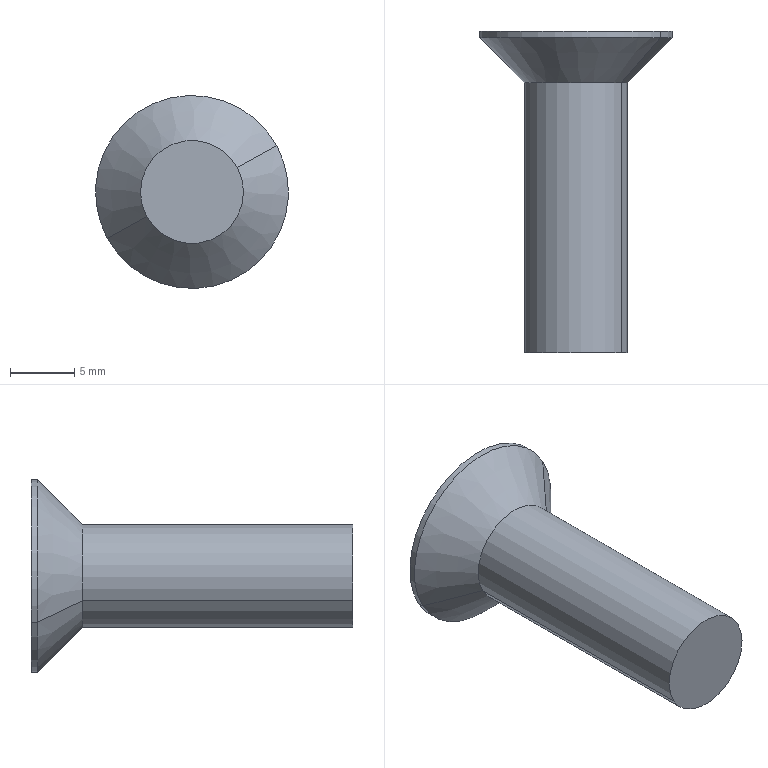Part | NX | features BREP 1 | 1 solid | 21 faces | box 15 x 25 x 15 mm | volume 1509 mm3 | plane 15 | cylinder 4 | cone 2 | commonest cylinder face diameters 8 x2 15 x2
STEP:
#1=CARTESIAN_POINT('',(3.51,31.308,1.918));
#2=VERTEX_POINT('',#1);
#3=CARTESIAN_POINT('',(-3.51,31.308,-1.918));
#4=VERTEX_POINT('',#3);
#5=CARTESIAN_POINT('',(0.,31.308,0.));
#6=DIRECTION('',(0.,-1.,0.));
#7=DIRECTION('',(1.,0.,0.));
#8=AXIS2_PLACEMENT_3D('',#5,#6,#7);
#9=CIRCLE('',#8,4.);
#10=EDGE_CURVE('',#2,#4,#9,.T.);
#11=ORIENTED_EDGE('',*,*,#10,.F.);
#12=CARTESIAN_POINT('',(3.51,52.308,1.918));
#13=VERTEX_POINT('',#12);
#14=CARTESIAN_POINT('',(3.51,41.808,1.918));
#15=DIRECTION('',(0.,-1.,0.));
#16=VECTOR('',#15,1000.);
#17=LINE('',#14,#16);
#18=EDGE_CURVE('',#2,#13,#17,.F.);
#19=ORIENTED_EDGE('',*,*,#18,.T.);
#20=CARTESIAN_POINT('',(-3.51,52.308,-1.918));
#21=VERTEX_POINT('',#20);
#22=CARTESIAN_POINT('',(0.,52.308,0.));
#23=DIRECTION('',(0.,1.,0.));
#24=DIRECTION('',(1.,0.,0.));
#25=AXIS2_PLACEMENT_3D('',#22,#23,#24);
#26=CIRCLE('',#25,4.);
#27=EDGE_CURVE('',#21,#13,#26,.T.);
#28=ORIENTED_EDGE('',*,*,#27,.F.);
#29=CARTESIAN_POINT('',(-3.51,41.808,-1.918));
#30=DIRECTION('',(0.,-1.,0.));
#31=VECTOR('',#30,1000.);
#32=LINE('',#29,#31);
#33=EDGE_CURVE('',#4,#21,#32,.F.);
#34=ORIENTED_EDGE('',*,*,#33,.F.);
#35=EDGE_LOOP('',(#11,#19,#28,#34));
#36=FACE_BOUND('',#35,.T.);
#37=CARTESIAN_POINT('',(0.,43.808,0.));
#38=DIRECTION('',(0.,-1.,0.));
#39=DIRECTION('',(0.8776,0.,0.4794));
#40=AXIS2_PLACEMENT_3D('',#37,#38,#39);
#41=CYLINDRICAL_SURFACE('',#40,4.);
#42=ADVANCED_FACE('',(#36),#41,.T.);
#43=CARTESIAN_POINT('',(0.,31.308,0.));
#44=DIRECTION('',(0.,-1.,0.));
#45=DIRECTION('',(1.,0.,0.));
#46=AXIS2_PLACEMENT_3D('',#43,#44,#45);
#47=CIRCLE('',#46,4.);
#48=EDGE_CURVE('',#4,#2,#47,.T.);
#49=ORIENTED_EDGE('',*,*,#48,.F.);
#50=ORIENTED_EDGE('',*,*,#33,.T.);
#51=CARTESIAN_POINT('',(0.,52.308,0.));
#52=DIRECTION('',(0.,1.,0.));
#53=DIRECTION('',(1.,0.,0.));
#54=AXIS2_PLACEMENT_3D('',#51,#52,#53);
#55=CIRCLE('',#54,4.);
#56=EDGE_CURVE('',#13,#21,#55,.T.);
#57=ORIENTED_EDGE('',*,*,#56,.F.);
#58=ORIENTED_EDGE('',*,*,#18,.F.);
#59=EDGE_LOOP('',(#49,#50,#57,#58));
#60=FACE_BOUND('',#59,.T.);
#61=CARTESIAN_POINT('',(0.,43.808,0.));
#62=DIRECTION('',(0.,-1.,0.));
#63=DIRECTION('',(0.8776,0.,0.4794));
#64=AXIS2_PLACEMENT_3D('',#61,#62,#63);
#65=CYLINDRICAL_SURFACE('',#64,4.);
#66=ADVANCED_FACE('',(#60),#65,.T.);
#67=ORIENTED_EDGE('',*,*,#27,.T.);
#68=CARTESIAN_POINT('',(6.582,55.808,3.596));
#69=VERTEX_POINT('',#68);
#70=CARTESIAN_POINT('',(5.046,54.058,2.757));
#71=DIRECTION('',(0.6205,0.7071,0.339));
#72=VECTOR('',#71,1000.);
#73=LINE('',#70,#72);
#74=EDGE_CURVE('',#69,#13,#73,.F.);
#75=ORIENTED_EDGE('',*,*,#74,.F.);
#76=CARTESIAN_POINT('',(-6.582,55.808,-3.596));
#77=VERTEX_POINT('',#76);
#78=CARTESIAN_POINT('',(0.,55.808,0.));
#79=DIRECTION('',(0.,-1.,0.));
#80=DIRECTION('',(1.,0.,0.));
#81=AXIS2_PLACEMENT_3D('',#78,#79,#80);
#82=CIRCLE('',#81,7.5);
#83=EDGE_CURVE('',#69,#77,#82,.T.);
#84=ORIENTED_EDGE('',*,*,#83,.T.);
#85=CARTESIAN_POINT('',(-5.046,54.058,-2.757));
#86=DIRECTION('',(-0.6205,0.7071,-0.339));
#87=VECTOR('',#86,1000.);
#88=LINE('',#85,#87);
#89=EDGE_CURVE('',#77,#21,#88,.F.);
#90=ORIENTED_EDGE('',*,*,#89,.T.);
#91=EDGE_LOOP('',(#67,#75,#84,#90));
#92=FACE_BOUND('',#91,.T.);
#93=CARTESIAN_POINT('',(0.,52.308,0.));
#94=DIRECTION('',(0.,1.,0.));
#95=DIRECTION('',(0.8776,0.,0.4794));
#96=AXIS2_PLACEMENT_3D('',#93,#94,#95);
#97=CONICAL_SURFACE('',#96,4.,0.7854);
#98=ADVANCED_FACE('',(#92),#97,.T.);
#99=ORIENTED_EDGE('',*,*,#56,.T.);
#100=ORIENTED_EDGE('',*,*,#89,.F.);
#101=CARTESIAN_POINT('',(0.,55.808,0.));
#102=DIRECTION('',(0.,-1.,0.));
#103=DIRECTION('',(1.,0.,0.));
#104=AXIS2_PLACEMENT_3D('',#101,#102,#103);
#105=CIRCLE('',#104,7.5);
#106=EDGE_CURVE('',#77,#69,#105,.T.);
#107=ORIENTED_EDGE('',*,*,#106,.T.);
#108=ORIENTED_EDGE('',*,*,#74,.T.);
#109=EDGE_LOOP('',(#99,#100,#107,#108));
#110=FACE_BOUND('',#109,.T.);
#111=CARTESIAN_POINT('',(0.,52.308,0.));
#112=DIRECTION('',(0.,1.,0.));
#113=DIRECTION('',(0.8776,0.,0.4794));
#114=AXIS2_PLACEMENT_3D('',#111,#112,#113);
#115=CONICAL_SURFACE('',#114,4.,0.7854);
#116=ADVANCED_FACE('',(#110),#115,.T.);
#117=ORIENTED_EDGE('',*,*,#83,.F.);
#118=CARTESIAN_POINT('',(6.582,56.308,3.596));
#119=VERTEX_POINT('',#118);
#120=CARTESIAN_POINT('',(6.582,56.058,3.596));
#121=DIRECTION('',(0.,-1.,0.));
#122=VECTOR('',#121,1000.);
#123=LINE('',#120,#122);
#124=EDGE_CURVE('',#69,#119,#123,.F.);
#125=ORIENTED_EDGE('',*,*,#124,.T.);
#126=CARTESIAN_POINT('',(-6.582,56.308,-3.596));
#127=VERTEX_POINT('',#126);
#128=CARTESIAN_POINT('',(0.,56.308,0.));
#129=DIRECTION('',(0.,-1.,0.));
#130=DIRECTION('',(1.,0.,0.));
#131=AXIS2_PLACEMENT_3D('',#128,#129,#130);
#132=CIRCLE('',#131,7.5);
#133=EDGE_CURVE('',#119,#127,#132,.T.);
#134=ORIENTED_EDGE('',*,*,#133,.T.);
#135=CARTESIAN_POINT('',(-6.582,56.058,-3.596));
#136=DIRECTION('',(0.,-1.,0.));
#137=VECTOR('',#136,1000.);
#138=LINE('',#135,#137);
#139=EDGE_CURVE('',#77,#127,#138,.F.);
#140=ORIENTED_EDGE('',*,*,#139,.F.);
#141=EDGE_LOOP('',(#117,#125,#134,#140));
#142=FACE_BOUND('',#141,.T.);
#143=CARTESIAN_POINT('',(0.,43.808,0.));
#144=DIRECTION('',(0.,-1.,0.));
#145=DIRECTION('',(0.8776,0.,0.4794));
#146=AXIS2_PLACEMENT_3D('',#143,#144,#145);
#147=CYLINDRICAL_SURFACE('',#146,7.5);
#148=ADVANCED_FACE('',(#142),#147,.T.);
#149=ORIENTED_EDGE('',*,*,#106,.F.);
#150=ORIENTED_EDGE('',*,*,#139,.T.);
#151=CARTESIAN_POINT('',(0.,56.308,0.));
#152=DIRECTION('',(0.,-1.,0.));
#153=DIRECTION('',(1.,0.,0.));
#154=AXIS2_PLACEMENT_3D('',#151,#152,#153);
#155=CIRCLE('',#154,7.5);
#156=EDGE_CURVE('',#127,#119,#155,.T.);
#157=ORIENTED_EDGE('',*,*,#156,.T.);
#158=ORIENTED_EDGE('',*,*,#124,.F.);
#159=EDGE_LOOP('',(#149,#150,#157,#158));
#160=FACE_BOUND('',#159,.T.);
#161=CARTESIAN_POINT('',(0.,43.808,0.));
#162=DIRECTION('',(0.,-1.,0.));
#163=DIRECTION('',(0.8776,0.,0.4794));
#164=AXIS2_PLACEMENT_3D('',#161,#162,#163);
#165=CYLINDRICAL_SURFACE('',#164,7.5);
#166=ADVANCED_FACE('',(#160),#165,.T.);
#167=ORIENTED_EDGE('',*,*,#10,.T.);
#168=ORIENTED_EDGE('',*,*,#48,.T.);
#169=EDGE_LOOP('',(#167,#168));
#170=FACE_BOUND('',#169,.T.);
#171=CARTESIAN_POINT('',(4.,31.308,0.));
#172=DIRECTION('',(0.,-1.,0.));
#173=DIRECTION('',(1.,0.,0.));
#174=AXIS2_PLACEMENT_3D('',#171,#172,#173);
#175=PLANE('',#174);
#176=ADVANCED_FACE('',(#170),#175,.T.);
#177=CARTESIAN_POINT('',(1.,56.308,2.));
#178=VERTEX_POINT('',#177);
#179=CARTESIAN_POINT('',(1.,56.308,1.));
#180=VERTEX_POINT('',#179);
#181=CARTESIAN_POINT('',(1.,56.308,1.5));
#182=DIRECTION('',(0.,0.,-1.));
#183=VECTOR('',#182,1000.);
#184=LINE('',#181,#183);
#185=EDGE_CURVE('',#178,#180,#184,.T.);
#186=ORIENTED_EDGE('',*,*,#185,.F.);
#187=CARTESIAN_POINT('',(-1.,56.308,2.));
#188=VERTEX_POINT('',#187);
#189=CARTESIAN_POINT('',(0.,56.308,2.));
#190=DIRECTION('',(-1.,0.,0.));
#191=VECTOR('',#190,1000.);
#192=LINE('',#189,#191);
#193=EDGE_CURVE('',#178,#188,#192,.T.);
#194=ORIENTED_EDGE('',*,*,#193,.T.);
#195=CARTESIAN_POINT('',(-1.,56.308,1.));
#196=VERTEX_POINT('',#195);
#197=CARTESIAN_POINT('',(-1.,56.308,1.5));
#198=DIRECTION('',(0.,0.,1.));
#199=VECTOR('',#198,1000.);
#200=LINE('',#197,#199);
#201=EDGE_CURVE('',#196,#188,#200,.T.);
#202=ORIENTED_EDGE('',*,*,#201,.F.);
#203=CARTESIAN_POINT('',(-2.,56.308,1.));
#204=VERTEX_POINT('',#203);
#205=CARTESIAN_POINT('',(-1.5,56.308,1.));
#206=DIRECTION('',(-1.,0.,0.));
#207=VECTOR('',#206,1000.);
#208=LINE('',#205,#207);
#209=EDGE_CURVE('',#196,#204,#208,.T.);
#210=ORIENTED_EDGE('',*,*,#209,.T.);
#211=CARTESIAN_POINT('',(-2.,56.308,-1.));
#212=VERTEX_POINT('',#211);
#213=CARTESIAN_POINT('',(-2.,56.308,0.));
#214=DIRECTION('',(0.,0.,1.));
#215=VECTOR('',#214,1000.);
#216=LINE('',#213,#215);
#217=EDGE_CURVE('',#212,#204,#216,.T.);
#218=ORIENTED_EDGE('',*,*,#217,.F.);
#219=CARTESIAN_POINT('',(-1.,56.308,-1.));
#220=VERTEX_POINT('',#219);
#221=CARTESIAN_POINT('',(-1.5,56.308,-1.));
#222=DIRECTION('',(1.,0.,0.));
#223=VECTOR('',#222,1000.);
#224=LINE('',#221,#223);
#225=EDGE_CURVE('',#212,#220,#224,.T.);
#226=ORIENTED_EDGE('',*,*,#225,.T.);
#227=CARTESIAN_POINT('',(-1.,56.308,-2.));
#228=VERTEX_POINT('',#227);
#229=CARTESIAN_POINT('',(-1.,56.308,-1.5));
#230=DIRECTION('',(0.,0.,1.));
#231=VECTOR('',#230,1000.);
#232=LINE('',#229,#231);
#233=EDGE_CURVE('',#228,#220,#232,.T.);
#234=ORIENTED_EDGE('',*,*,#233,.F.);
#235=CARTESIAN_POINT('',(1.,56.308,-2.));
#236=VERTEX_POINT('',#235);
#237=CARTESIAN_POINT('',(0.,56.308,-2.));
#238=DIRECTION('',(1.,0.,0.));
#239=VECTOR('',#238,1000.);
#240=LINE('',#237,#239);
#241=EDGE_CURVE('',#228,#236,#240,.T.);
#242=ORIENTED_EDGE('',*,*,#241,.T.);
#243=CARTESIAN_POINT('',(1.,56.308,-1.));
#244=VERTEX_POINT('',#243);
#245=CARTESIAN_POINT('',(1.,56.308,-1.5));
#246=DIRECTION('',(0.,0.,-1.));
#247=VECTOR('',#246,1000.);
#248=LINE('',#245,#247);
#249=EDGE_CURVE('',#244,#236,#248,.T.);
#250=ORIENTED_EDGE('',*,*,#249,.F.);
#251=CARTESIAN_POINT('',(2.,56.308,-1.));
#252=VERTEX_POINT('',#251);
#253=CARTESIAN_POINT('',(1.5,56.308,-1.));
#254=DIRECTION('',(1.,0.,0.));
#255=VECTOR('',#254,1000.);
#256=LINE('',#253,#255);
#257=EDGE_CURVE('',#244,#252,#256,.T.);
#258=ORIENTED_EDGE('',*,*,#257,.T.);
#259=CARTESIAN_POINT('',(2.,56.308,1.));
#260=VERTEX_POINT('',#259);
#261=CARTESIAN_POINT('',(2.,56.308,0.));
#262=DIRECTION('',(0.,0.,-1.));
#263=VECTOR('',#262,1000.);
#264=LINE('',#261,#263);
#265=EDGE_CURVE('',#260,#252,#264,.T.);
#266=ORIENTED_EDGE('',*,*,#265,.F.);
#267=CARTESIAN_POINT('',(1.5,56.308,1.));
#268=DIRECTION('',(-1.,0.,0.));
#269=VECTOR('',#268,1000.);
#270=LINE('',#267,#269);
#271=EDGE_CURVE('',#260,#180,#270,.T.);
#272=ORIENTED_EDGE('',*,*,#271,.T.);
#273=EDGE_LOOP('',(#186,#194,#202,#210,#218,#226,#234,#242,#250,#258,#266,#272));
#274=FACE_BOUND('',#273,.T.);
#275=ORIENTED_EDGE('',*,*,#133,.F.);
#276=ORIENTED_EDGE('',*,*,#156,.F.);
#277=EDGE_LOOP('',(#275,#276));
#278=FACE_BOUND('',#277,.T.);
#279=CARTESIAN_POINT('',(0.,56.308,0.));
#280=DIRECTION('',(0.,-1.,0.));
#281=DIRECTION('',(1.,0.,0.));
#282=AXIS2_PLACEMENT_3D('',#279,#280,#281);
#283=PLANE('',#282);
#284=ADVANCED_FACE('',(#274,#278),#283,.F.);
#285=CARTESIAN_POINT('',(-1.,55.508,2.));
#286=VERTEX_POINT('',#285);
#287=CARTESIAN_POINT('',(-1.,55.908,2.));
#288=DIRECTION('',(0.,-1.,0.));
#289=VECTOR('',#288,1000.);
#290=LINE('',#287,#289);
#291=EDGE_CURVE('',#188,#286,#290,.T.);
#292=ORIENTED_EDGE('',*,*,#291,.F.);
#293=ORIENTED_EDGE('',*,*,#193,.F.);
#294=CARTESIAN_POINT('',(1.,55.508,2.));
#295=VERTEX_POINT('',#294);
#296=CARTESIAN_POINT('',(1.,55.908,2.));
#297=DIRECTION('',(0.,-1.,0.));
#298=VECTOR('',#297,1000.);
#299=LINE('',#296,#298);
#300=EDGE_CURVE('',#178,#295,#299,.T.);
#301=ORIENTED_EDGE('',*,*,#300,.T.);
#302=CARTESIAN_POINT('',(0.,55.508,2.));
#303=DIRECTION('',(-1.,0.,0.));
#304=VECTOR('',#303,1000.);
#305=LINE('',#302,#304);
#306=EDGE_CURVE('',#295,#286,#305,.T.);
#307=ORIENTED_EDGE('',*,*,#306,.T.);
#308=EDGE_LOOP('',(#292,#293,#301,#307));
#309=FACE_BOUND('',#308,.T.);
#310=CARTESIAN_POINT('',(1.,56.308,2.));
#311=DIRECTION('',(0.,0.,1.));
#312=DIRECTION('',(-1.,0.,0.));
#313=AXIS2_PLACEMENT_3D('',#310,#311,#312);
#314=PLANE('',#313);
#315=ADVANCED_FACE('',(#309),#314,.F.);
#316=CARTESIAN_POINT('',(-1.,55.508,1.));
#317=VERTEX_POINT('',#316);
#318=CARTESIAN_POINT('',(-1.,55.908,1.));
#319=DIRECTION('',(0.,-1.,0.));
#320=VECTOR('',#319,1000.);
#321=LINE('',#318,#320);
#322=EDGE_CURVE('',#196,#317,#321,.T.);
#323=ORIENTED_EDGE('',*,*,#322,.F.);
#324=ORIENTED_EDGE('',*,*,#201,.T.);
#325=ORIENTED_EDGE('',*,*,#291,.T.);
#326=CARTESIAN_POINT('',(-1.,55.508,1.5));
#327=DIRECTION('',(0.,0.,1.));
#328=VECTOR('',#327,1000.);
#329=LINE('',#326,#328);
#330=EDGE_CURVE('',#317,#286,#329,.T.);
#331=ORIENTED_EDGE('',*,*,#330,.F.);
#332=EDGE_LOOP('',(#323,#324,#325,#331));
#333=FACE_BOUND('',#332,.T.);
#334=CARTESIAN_POINT('',(-1.,56.308,-2.));
#335=DIRECTION('',(1.,0.,0.));
#336=DIRECTION('',(0.,0.,1.));
#337=AXIS2_PLACEMENT_3D('',#334,#335,#336);
#338=PLANE('',#337);
#339=ADVANCED_FACE('',(#333),#338,.T.);
#340=CARTESIAN_POINT('',(-2.,55.508,1.));
#341=VERTEX_POINT('',#340);
#342=CARTESIAN_POINT('',(-2.,55.908,1.));
#343=DIRECTION('',(0.,-1.,0.));
#344=VECTOR('',#343,1000.);
#345=LINE('',#342,#344);
#346=EDGE_CURVE('',#204,#341,#345,.T.);
#347=ORIENTED_EDGE('',*,*,#346,.F.);
#348=ORIENTED_EDGE('',*,*,#209,.F.);
#349=ORIENTED_EDGE('',*,*,#322,.T.);
#350=CARTESIAN_POINT('',(-1.5,55.508,1.));
#351=DIRECTION('',(-1.,0.,0.));
#352=VECTOR('',#351,1000.);
#353=LINE('',#350,#352);
#354=EDGE_CURVE('',#317,#341,#353,.T.);
#355=ORIENTED_EDGE('',*,*,#354,.T.);
#356=EDGE_LOOP('',(#347,#348,#349,#355));
#357=FACE_BOUND('',#356,.T.);
#358=CARTESIAN_POINT('',(-1.,56.308,1.));
#359=DIRECTION('',(0.,0.,1.));
#360=DIRECTION('',(-1.,0.,0.));
#361=AXIS2_PLACEMENT_3D('',#358,#359,#360);
#362=PLANE('',#361);
#363=ADVANCED_FACE('',(#357),#362,.F.);
#364=CARTESIAN_POINT('',(-2.,55.508,-1.));
#365=VERTEX_POINT('',#364);
#366=CARTESIAN_POINT('',(-2.,55.908,-1.));
#367=DIRECTION('',(0.,-1.,0.));
#368=VECTOR('',#367,1000.);
#369=LINE('',#366,#368);
#370=EDGE_CURVE('',#212,#365,#369,.T.);
#371=ORIENTED_EDGE('',*,*,#370,.F.);
#372=ORIENTED_EDGE('',*,*,#217,.T.);
#373=ORIENTED_EDGE('',*,*,#346,.T.);
#374=CARTESIAN_POINT('',(-2.,55.508,0.));
#375=DIRECTION('',(0.,0.,1.));
#376=VECTOR('',#375,1000.);
#377=LINE('',#374,#376);
#378=EDGE_CURVE('',#365,#341,#377,.T.);
#379=ORIENTED_EDGE('',*,*,#378,.F.);
#380=EDGE_LOOP('',(#371,#372,#373,#379));
#381=FACE_BOUND('',#380,.T.);
#382=CARTESIAN_POINT('',(-2.,56.308,-1.));
#383=DIRECTION('',(1.,0.,0.));
#384=DIRECTION('',(0.,0.,1.));
#385=AXIS2_PLACEMENT_3D('',#382,#383,#384);
#386=PLANE('',#385);
#387=ADVANCED_FACE('',(#381),#386,.T.);
#388=CARTESIAN_POINT('',(-1.,55.508,-1.));
#389=VERTEX_POINT('',#388);
#390=CARTESIAN_POINT('',(-1.,55.908,-1.));
#391=DIRECTION('',(0.,-1.,0.));
#392=VECTOR('',#391,1000.);
#393=LINE('',#390,#392);
#394=EDGE_CURVE('',#220,#389,#393,.T.);
#395=ORIENTED_EDGE('',*,*,#394,.F.);
#396=ORIENTED_EDGE('',*,*,#225,.F.);
#397=ORIENTED_EDGE('',*,*,#370,.T.);
#398=CARTESIAN_POINT('',(-1.5,55.508,-1.));
#399=DIRECTION('',(1.,0.,0.));
#400=VECTOR('',#399,1000.);
#401=LINE('',#398,#400);
#402=EDGE_CURVE('',#365,#389,#401,.T.);
#403=ORIENTED_EDGE('',*,*,#402,.T.);
#404=EDGE_LOOP('',(#395,#396,#397,#403));
#405=FACE_BOUND('',#404,.T.);
#406=CARTESIAN_POINT('',(1.,56.308,-1.));
#407=DIRECTION('',(0.,0.,-1.));
#408=DIRECTION('',(1.,0.,0.));
#409=AXIS2_PLACEMENT_3D('',#406,#407,#408);
#410=PLANE('',#409);
#411=ADVANCED_FACE('',(#405),#410,.F.);
#412=CARTESIAN_POINT('',(-1.,55.508,-2.));
#413=VERTEX_POINT('',#412);
#414=CARTESIAN_POINT('',(-1.,55.908,-2.));
#415=DIRECTION('',(0.,-1.,0.));
#416=VECTOR('',#415,1000.);
#417=LINE('',#414,#416);
#418=EDGE_CURVE('',#228,#413,#417,.T.);
#419=ORIENTED_EDGE('',*,*,#418,.F.);
#420=ORIENTED_EDGE('',*,*,#233,.T.);
#421=ORIENTED_EDGE('',*,*,#394,.T.);
#422=CARTESIAN_POINT('',(-1.,55.508,-1.5));
#423=DIRECTION('',(0.,0.,1.));
#424=VECTOR('',#423,1000.);
#425=LINE('',#422,#424);
#426=EDGE_CURVE('',#413,#389,#425,.T.);
#427=ORIENTED_EDGE('',*,*,#426,.F.);
#428=EDGE_LOOP('',(#419,#420,#421,#427));
#429=FACE_BOUND('',#428,.T.);
#430=CARTESIAN_POINT('',(-1.,56.308,-2.));
#431=DIRECTION('',(1.,0.,0.));
#432=DIRECTION('',(0.,0.,1.));
#433=AXIS2_PLACEMENT_3D('',#430,#431,#432);
#434=PLANE('',#433);
#435=ADVANCED_FACE('',(#429),#434,.T.);
#436=CARTESIAN_POINT('',(1.,55.508,-2.));
#437=VERTEX_POINT('',#436);
#438=CARTESIAN_POINT('',(1.,55.908,-2.));
#439=DIRECTION('',(0.,-1.,0.));
#440=VECTOR('',#439,1000.);
#441=LINE('',#438,#440);
#442=EDGE_CURVE('',#236,#437,#441,.T.);
#443=ORIENTED_EDGE('',*,*,#442,.F.);
#444=ORIENTED_EDGE('',*,*,#241,.F.);
#445=ORIENTED_EDGE('',*,*,#418,.T.);
#446=CARTESIAN_POINT('',(0.,55.508,-2.));
#447=DIRECTION('',(1.,0.,0.));
#448=VECTOR('',#447,1000.);
#449=LINE('',#446,#448);
#450=EDGE_CURVE('',#413,#437,#449,.T.);
#451=ORIENTED_EDGE('',*,*,#450,.T.);
#452=EDGE_LOOP('',(#443,#444,#445,#451));
#453=FACE_BOUND('',#452,.T.);
#454=CARTESIAN_POINT('',(-1.,56.308,-2.));
#455=DIRECTION('',(0.,0.,-1.));
#456=DIRECTION('',(1.,0.,0.));
#457=AXIS2_PLACEMENT_3D('',#454,#455,#456);
#458=PLANE('',#457);
#459=ADVANCED_FACE('',(#453),#458,.F.);
#460=CARTESIAN_POINT('',(1.,55.508,-1.));
#461=VERTEX_POINT('',#460);
#462=CARTESIAN_POINT('',(1.,55.908,-1.));
#463=DIRECTION('',(0.,-1.,0.));
#464=VECTOR('',#463,1000.);
#465=LINE('',#462,#464);
#466=EDGE_CURVE('',#244,#461,#465,.T.);
#467=ORIENTED_EDGE('',*,*,#466,.F.);
#468=ORIENTED_EDGE('',*,*,#249,.T.);
#469=ORIENTED_EDGE('',*,*,#442,.T.);
#470=CARTESIAN_POINT('',(1.,55.508,-1.5));
#471=DIRECTION('',(0.,0.,-1.));
#472=VECTOR('',#471,1000.);
#473=LINE('',#470,#472);
#474=EDGE_CURVE('',#461,#437,#473,.T.);
#475=ORIENTED_EDGE('',*,*,#474,.F.);
#476=EDGE_LOOP('',(#467,#468,#469,#475));
#477=FACE_BOUND('',#476,.T.);
#478=CARTESIAN_POINT('',(1.,56.308,-1.));
#479=DIRECTION('',(-1.,0.,0.));
#480=DIRECTION('',(0.,0.,-1.));
#481=AXIS2_PLACEMENT_3D('',#478,#479,#480);
#482=PLANE('',#481);
#483=ADVANCED_FACE('',(#477),#482,.T.);
#484=ORIENTED_EDGE('',*,*,#300,.F.);
#485=ORIENTED_EDGE('',*,*,#185,.T.);
#486=CARTESIAN_POINT('',(1.,55.508,1.));
#487=VERTEX_POINT('',#486);
#488=CARTESIAN_POINT('',(1.,55.908,1.));
#489=DIRECTION('',(0.,-1.,0.));
#490=VECTOR('',#489,1000.);
#491=LINE('',#488,#490);
#492=EDGE_CURVE('',#180,#487,#491,.T.);
#493=ORIENTED_EDGE('',*,*,#492,.T.);
#494=CARTESIAN_POINT('',(1.,55.508,1.5));
#495=DIRECTION('',(0.,0.,-1.));
#496=VECTOR('',#495,1000.);
#497=LINE('',#494,#496);
#498=EDGE_CURVE('',#295,#487,#497,.T.);
#499=ORIENTED_EDGE('',*,*,#498,.F.);
#500=EDGE_LOOP('',(#484,#485,#493,#499));
#501=FACE_BOUND('',#500,.T.);
#502=CARTESIAN_POINT('',(1.,56.308,-1.));
#503=DIRECTION('',(-1.,0.,0.));
#504=DIRECTION('',(0.,0.,-1.));
#505=AXIS2_PLACEMENT_3D('',#502,#503,#504);
#506=PLANE('',#505);
#507=ADVANCED_FACE('',(#501),#506,.T.);
#508=CARTESIAN_POINT('',(2.,55.508,1.));
#509=VERTEX_POINT('',#508);
#510=CARTESIAN_POINT('',(2.,55.508,-1.));
#511=VERTEX_POINT('',#510);
#512=CARTESIAN_POINT('',(2.,55.508,0.));
#513=DIRECTION('',(0.,0.,-1.));
#514=VECTOR('',#513,1000.);
#515=LINE('',#512,#514);
#516=EDGE_CURVE('',#509,#511,#515,.T.);
#517=ORIENTED_EDGE('',*,*,#516,.T.);
#518=CARTESIAN_POINT('',(1.5,55.508,-1.));
#519=DIRECTION('',(1.,0.,0.));
#520=VECTOR('',#519,1000.);
#521=LINE('',#518,#520);
#522=EDGE_CURVE('',#461,#511,#521,.T.);
#523=ORIENTED_EDGE('',*,*,#522,.F.);
#524=ORIENTED_EDGE('',*,*,#474,.T.);
#525=ORIENTED_EDGE('',*,*,#450,.F.);
#526=ORIENTED_EDGE('',*,*,#426,.T.);
#527=ORIENTED_EDGE('',*,*,#402,.F.);
#528=ORIENTED_EDGE('',*,*,#378,.T.);
#529=ORIENTED_EDGE('',*,*,#354,.F.);
#530=ORIENTED_EDGE('',*,*,#330,.T.);
#531=ORIENTED_EDGE('',*,*,#306,.F.);
#532=ORIENTED_EDGE('',*,*,#498,.T.);
#533=CARTESIAN_POINT('',(1.5,55.508,1.));
#534=DIRECTION('',(-1.,0.,0.));
#535=VECTOR('',#534,1000.);
#536=LINE('',#533,#535);
#537=EDGE_CURVE('',#509,#487,#536,.T.);
#538=ORIENTED_EDGE('',*,*,#537,.F.);
#539=EDGE_LOOP('',(#517,#523,#524,#525,#526,#527,#528,#529,#530,#531,#532,#538));
#540=FACE_BOUND('',#539,.T.);
#541=CARTESIAN_POINT('',(0.,55.508,0.));
#542=DIRECTION('',(0.,1.,0.));
#543=DIRECTION('',(-1.,0.,0.));
#544=AXIS2_PLACEMENT_3D('',#541,#542,#543);
#545=PLANE('',#544);
#546=ADVANCED_FACE('',(#540),#545,.T.);
#547=CARTESIAN_POINT('',(2.,55.908,-1.));
#548=DIRECTION('',(0.,-1.,0.));
#549=VECTOR('',#548,1000.);
#550=LINE('',#547,#549);
#551=EDGE_CURVE('',#252,#511,#550,.T.);
#552=ORIENTED_EDGE('',*,*,#551,.F.);
#553=ORIENTED_EDGE('',*,*,#257,.F.);
#554=ORIENTED_EDGE('',*,*,#466,.T.);
#555=ORIENTED_EDGE('',*,*,#522,.T.);
#556=EDGE_LOOP('',(#552,#553,#554,#555));
#557=FACE_BOUND('',#556,.T.);
#558=CARTESIAN_POINT('',(1.,56.308,-1.));
#559=DIRECTION('',(0.,0.,-1.));
#560=DIRECTION('',(1.,0.,0.));
#561=AXIS2_PLACEMENT_3D('',#558,#559,#560);
#562=PLANE('',#561);
#563=ADVANCED_FACE('',(#557),#562,.F.);
#564=ORIENTED_EDGE('',*,*,#492,.F.);
#565=ORIENTED_EDGE('',*,*,#271,.F.);
#566=CARTESIAN_POINT('',(2.,55.908,1.));
#567=DIRECTION('',(0.,-1.,0.));
#568=VECTOR('',#567,1000.);
#569=LINE('',#566,#568);
#570=EDGE_CURVE('',#260,#509,#569,.T.);
#571=ORIENTED_EDGE('',*,*,#570,.T.);
#572=ORIENTED_EDGE('',*,*,#537,.T.);
#573=EDGE_LOOP('',(#564,#565,#571,#572));
#574=FACE_BOUND('',#573,.T.);
#575=CARTESIAN_POINT('',(-1.,56.308,1.));
#576=DIRECTION('',(0.,0.,1.));
#577=DIRECTION('',(-1.,0.,0.));
#578=AXIS2_PLACEMENT_3D('',#575,#576,#577);
#579=PLANE('',#578);
#580=ADVANCED_FACE('',(#574),#579,.F.);
#581=ORIENTED_EDGE('',*,*,#570,.F.);
#582=ORIENTED_EDGE('',*,*,#265,.T.);
#583=ORIENTED_EDGE('',*,*,#551,.T.);
#584=ORIENTED_EDGE('',*,*,#516,.F.);
#585=EDGE_LOOP('',(#581,#582,#583,#584));
#586=FACE_BOUND('',#585,.T.);
#587=CARTESIAN_POINT('',(2.,56.308,1.));
#588=DIRECTION('',(-1.,0.,0.));
#589=DIRECTION('',(0.,0.,-1.));
#590=AXIS2_PLACEMENT_3D('',#587,#588,#589);
#591=PLANE('',#590);
#592=ADVANCED_FACE('',(#586),#591,.T.);
#593=CLOSED_SHELL('',(#42,#66,#98,#116,#148,#166,#176,#284,#315,#339,#363,#387,#411,#435,#459,#483,#507,#546,#563,#580,#592));
#594=MANIFOLD_SOLID_BREP('',#593);
#595=(LENGTH_UNIT()NAMED_UNIT(*)SI_UNIT(.MILLI.,.METRE.));
#596=UNCERTAINTY_MEASURE_WITH_UNIT(LENGTH_MEASURE(0.00001),#595,'','');
#597=(NAMED_UNIT(*)PLANE_ANGLE_UNIT()SI_UNIT($,.RADIAN.));
#598=(NAMED_UNIT(*)SI_UNIT($,.STERADIAN.)SOLID_ANGLE_UNIT());
#599=(GEOMETRIC_REPRESENTATION_CONTEXT(3)GLOBAL_UNCERTAINTY_ASSIGNED_CONTEXT((#596))GLOBAL_UNIT_ASSIGNED_CONTEXT((#595,#597,#598))REPRESENTATION_CONTEXT('',''));
#600=ADVANCED_BREP_SHAPE_REPRESENTATION('',(#594),#599);